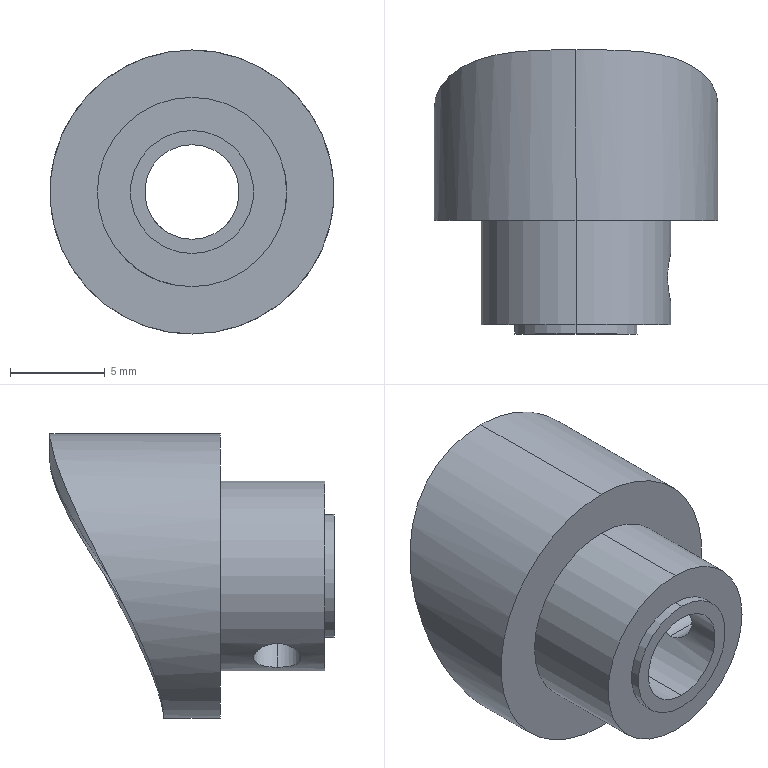Part | SolidWorks | features ICE 5, CirPattern 1, Emboss 1, Extrusion 1, HoleWzd 1, RefAxis 1 | 1 solid | 22 faces | box 15 x 15 x 15 mm | volume 872.889 mm3 | cylinder 14 | plane 6 | spline 2 | commonest cylinder face diameters 2.5 x4 5 x2 6.5 x2 10 x2 12 x2 15 x2